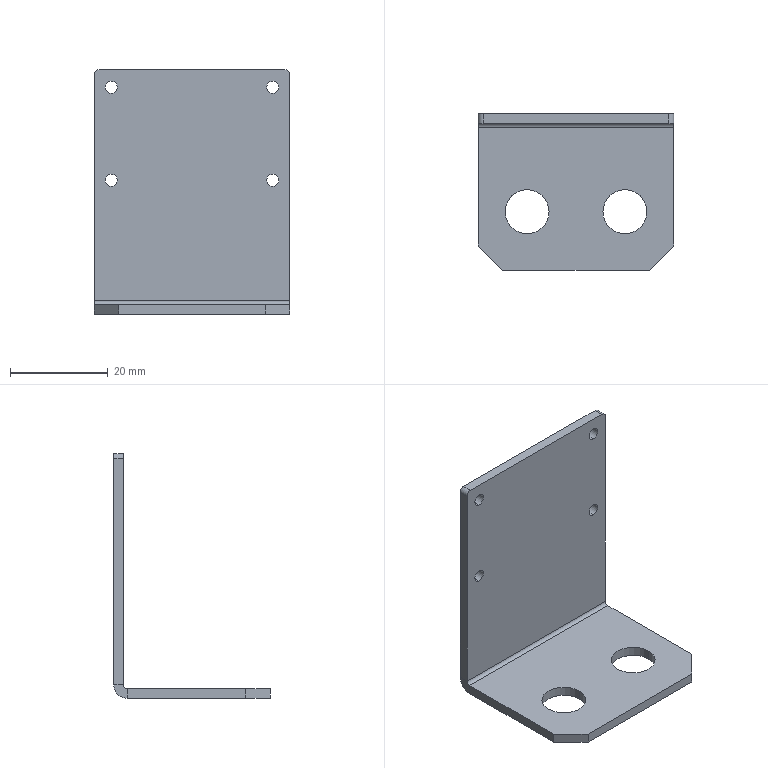Part | SolidWorks | features BaseBody 1 | 1 solid | 30 faces | box 40 x 32 x 50 mm | volume 5996 mm3 | cylinder 16 | plane 14 | commonest cylinder face diameters 2.5 x8 9 x4 2 x2 1.473 x1 5.473 x1
STEP:
#1=CARTESIAN_POINT('',(16.525,15.,24.15));
#2=VERTEX_POINT('',#1);
#3=CARTESIAN_POINT('',(16.525,15.,26.65));
#4=VERTEX_POINT('',#3);
#5=CARTESIAN_POINT('',(16.525,15.,25.4));
#6=DIRECTION('',(0.,1.,0.));
#7=DIRECTION('',(0.,0.,1.));
#8=AXIS2_PLACEMENT_3D('',#5,#6,#7);
#9=CIRCLE('',#8,1.25);
#10=EDGE_CURVE('',#2,#4,#9,.T.);
#11=ORIENTED_EDGE('',*,*,#10,.F.);
#12=CARTESIAN_POINT('',(16.525,17.,24.15));
#13=VERTEX_POINT('',#12);
#14=CARTESIAN_POINT('',(16.525,17.,24.15));
#15=DIRECTION('',(0.,1.,0.));
#16=VECTOR('',#15,1000.);
#17=LINE('',#14,#16);
#18=EDGE_CURVE('',#2,#13,#17,.T.);
#19=ORIENTED_EDGE('',*,*,#18,.T.);
#20=CARTESIAN_POINT('',(16.525,17.,26.65));
#21=VERTEX_POINT('',#20);
#22=CARTESIAN_POINT('',(16.525,17.,25.4));
#23=DIRECTION('',(0.,1.,0.));
#24=DIRECTION('',(0.,0.,1.));
#25=AXIS2_PLACEMENT_3D('',#22,#23,#24);
#26=CIRCLE('',#25,1.25);
#27=EDGE_CURVE('',#13,#21,#26,.T.);
#28=ORIENTED_EDGE('',*,*,#27,.T.);
#29=CARTESIAN_POINT('',(16.525,17.,26.65));
#30=DIRECTION('',(0.,1.,0.));
#31=VECTOR('',#30,1000.);
#32=LINE('',#29,#31);
#33=EDGE_CURVE('',#4,#21,#32,.T.);
#34=ORIENTED_EDGE('',*,*,#33,.F.);
#35=EDGE_LOOP('',(#11,#19,#28,#34));
#36=FACE_OUTER_BOUND('',#35,.T.);
#37=CARTESIAN_POINT('',(16.525,17.,25.4));
#38=DIRECTION('',(0.,1.,0.));
#39=DIRECTION('',(0.,0.,1.));
#40=AXIS2_PLACEMENT_3D('',#37,#38,#39);
#41=CYLINDRICAL_SURFACE('',#40,1.25);
#42=ADVANCED_FACE('',(#36),#41,.F.);
#43=CARTESIAN_POINT('',(16.525,15.,43.15));
#44=VERTEX_POINT('',#43);
#45=CARTESIAN_POINT('',(16.525,15.,45.65));
#46=VERTEX_POINT('',#45);
#47=CARTESIAN_POINT('',(16.525,15.,44.4));
#48=DIRECTION('',(0.,1.,0.));
#49=DIRECTION('',(0.,0.,1.));
#50=AXIS2_PLACEMENT_3D('',#47,#48,#49);
#51=CIRCLE('',#50,1.25);
#52=EDGE_CURVE('',#44,#46,#51,.T.);
#53=ORIENTED_EDGE('',*,*,#52,.F.);
#54=CARTESIAN_POINT('',(16.525,17.,43.15));
#55=VERTEX_POINT('',#54);
#56=CARTESIAN_POINT('',(16.525,17.,43.15));
#57=DIRECTION('',(0.,1.,0.));
#58=VECTOR('',#57,1000.);
#59=LINE('',#56,#58);
#60=EDGE_CURVE('',#44,#55,#59,.T.);
#61=ORIENTED_EDGE('',*,*,#60,.T.);
#62=CARTESIAN_POINT('',(16.525,17.,45.65));
#63=VERTEX_POINT('',#62);
#64=CARTESIAN_POINT('',(16.525,17.,44.4));
#65=DIRECTION('',(0.,1.,0.));
#66=DIRECTION('',(0.,0.,1.));
#67=AXIS2_PLACEMENT_3D('',#64,#65,#66);
#68=CIRCLE('',#67,1.25);
#69=EDGE_CURVE('',#55,#63,#68,.T.);
#70=ORIENTED_EDGE('',*,*,#69,.T.);
#71=CARTESIAN_POINT('',(16.525,17.,45.65));
#72=DIRECTION('',(0.,1.,0.));
#73=VECTOR('',#72,1000.);
#74=LINE('',#71,#73);
#75=EDGE_CURVE('',#46,#63,#74,.T.);
#76=ORIENTED_EDGE('',*,*,#75,.F.);
#77=EDGE_LOOP('',(#53,#61,#70,#76));
#78=FACE_OUTER_BOUND('',#77,.T.);
#79=CARTESIAN_POINT('',(16.525,17.,44.4));
#80=DIRECTION('',(0.,1.,0.));
#81=DIRECTION('',(0.,0.,1.));
#82=AXIS2_PLACEMENT_3D('',#79,#80,#81);
#83=CYLINDRICAL_SURFACE('',#82,1.25);
#84=ADVANCED_FACE('',(#78),#83,.F.);
#85=CARTESIAN_POINT('',(-16.525,15.,43.15));
#86=VERTEX_POINT('',#85);
#87=CARTESIAN_POINT('',(-16.525,15.,45.65));
#88=VERTEX_POINT('',#87);
#89=CARTESIAN_POINT('',(-16.525,15.,44.4));
#90=DIRECTION('',(0.,1.,0.));
#91=DIRECTION('',(0.,0.,1.));
#92=AXIS2_PLACEMENT_3D('',#89,#90,#91);
#93=CIRCLE('',#92,1.25);
#94=EDGE_CURVE('',#86,#88,#93,.T.);
#95=ORIENTED_EDGE('',*,*,#94,.F.);
#96=CARTESIAN_POINT('',(-16.525,17.,43.15));
#97=VERTEX_POINT('',#96);
#98=CARTESIAN_POINT('',(-16.525,17.,43.15));
#99=DIRECTION('',(0.,1.,0.));
#100=VECTOR('',#99,1000.);
#101=LINE('',#98,#100);
#102=EDGE_CURVE('',#86,#97,#101,.T.);
#103=ORIENTED_EDGE('',*,*,#102,.T.);
#104=CARTESIAN_POINT('',(-16.525,17.,45.65));
#105=VERTEX_POINT('',#104);
#106=CARTESIAN_POINT('',(-16.525,17.,44.4));
#107=DIRECTION('',(0.,1.,0.));
#108=DIRECTION('',(0.,0.,1.));
#109=AXIS2_PLACEMENT_3D('',#106,#107,#108);
#110=CIRCLE('',#109,1.25);
#111=EDGE_CURVE('',#97,#105,#110,.T.);
#112=ORIENTED_EDGE('',*,*,#111,.T.);
#113=CARTESIAN_POINT('',(-16.525,17.,45.65));
#114=DIRECTION('',(0.,1.,0.));
#115=VECTOR('',#114,1000.);
#116=LINE('',#113,#115);
#117=EDGE_CURVE('',#88,#105,#116,.T.);
#118=ORIENTED_EDGE('',*,*,#117,.F.);
#119=EDGE_LOOP('',(#95,#103,#112,#118));
#120=FACE_OUTER_BOUND('',#119,.T.);
#121=CARTESIAN_POINT('',(-16.525,17.,44.4));
#122=DIRECTION('',(0.,1.,0.));
#123=DIRECTION('',(0.,0.,1.));
#124=AXIS2_PLACEMENT_3D('',#121,#122,#123);
#125=CYLINDRICAL_SURFACE('',#124,1.25);
#126=ADVANCED_FACE('',(#120),#125,.F.);
#127=CARTESIAN_POINT('',(-16.525,15.,24.15));
#128=VERTEX_POINT('',#127);
#129=CARTESIAN_POINT('',(-16.525,15.,26.65));
#130=VERTEX_POINT('',#129);
#131=CARTESIAN_POINT('',(-16.525,15.,25.4));
#132=DIRECTION('',(0.,1.,0.));
#133=DIRECTION('',(0.,0.,1.));
#134=AXIS2_PLACEMENT_3D('',#131,#132,#133);
#135=CIRCLE('',#134,1.25);
#136=EDGE_CURVE('',#128,#130,#135,.T.);
#137=ORIENTED_EDGE('',*,*,#136,.F.);
#138=CARTESIAN_POINT('',(-16.525,17.,24.15));
#139=VERTEX_POINT('',#138);
#140=CARTESIAN_POINT('',(-16.525,17.,24.15));
#141=DIRECTION('',(0.,1.,0.));
#142=VECTOR('',#141,1000.);
#143=LINE('',#140,#142);
#144=EDGE_CURVE('',#128,#139,#143,.T.);
#145=ORIENTED_EDGE('',*,*,#144,.T.);
#146=CARTESIAN_POINT('',(-16.525,17.,26.65));
#147=VERTEX_POINT('',#146);
#148=CARTESIAN_POINT('',(-16.525,17.,25.4));
#149=DIRECTION('',(0.,1.,0.));
#150=DIRECTION('',(0.,0.,1.));
#151=AXIS2_PLACEMENT_3D('',#148,#149,#150);
#152=CIRCLE('',#151,1.25);
#153=EDGE_CURVE('',#139,#147,#152,.T.);
#154=ORIENTED_EDGE('',*,*,#153,.T.);
#155=CARTESIAN_POINT('',(-16.525,17.,26.65));
#156=DIRECTION('',(0.,1.,0.));
#157=VECTOR('',#156,1000.);
#158=LINE('',#155,#157);
#159=EDGE_CURVE('',#130,#147,#158,.T.);
#160=ORIENTED_EDGE('',*,*,#159,.F.);
#161=EDGE_LOOP('',(#137,#145,#154,#160));
#162=FACE_OUTER_BOUND('',#161,.T.);
#163=CARTESIAN_POINT('',(-16.525,17.,25.4));
#164=DIRECTION('',(0.,1.,0.));
#165=DIRECTION('',(0.,0.,1.));
#166=AXIS2_PLACEMENT_3D('',#163,#164,#165);
#167=CYLINDRICAL_SURFACE('',#166,1.25);
#168=ADVANCED_FACE('',(#162),#167,.F.);
#169=CARTESIAN_POINT('',(-14.5,-3.,-2.));
#170=VERTEX_POINT('',#169);
#171=CARTESIAN_POINT('',(-5.5,-3.,-2.));
#172=VERTEX_POINT('',#171);
#173=CARTESIAN_POINT('',(-10.,-3.,-2.));
#174=DIRECTION('',(0.,0.,1.));
#175=DIRECTION('',(1.,0.,0.));
#176=AXIS2_PLACEMENT_3D('',#173,#174,#175);
#177=CIRCLE('',#176,4.5);
#178=EDGE_CURVE('',#170,#172,#177,.T.);
#179=ORIENTED_EDGE('',*,*,#178,.F.);
#180=CARTESIAN_POINT('',(-14.5,-3.,0.));
#181=VERTEX_POINT('',#180);
#182=CARTESIAN_POINT('',(-14.5,-3.,0.));
#183=DIRECTION('',(0.,0.,1.));
#184=VECTOR('',#183,1000.);
#185=LINE('',#182,#184);
#186=EDGE_CURVE('',#170,#181,#185,.T.);
#187=ORIENTED_EDGE('',*,*,#186,.T.);
#188=CARTESIAN_POINT('',(-5.5,-3.,0.));
#189=VERTEX_POINT('',#188);
#190=CARTESIAN_POINT('',(-10.,-3.,0.));
#191=DIRECTION('',(0.,0.,1.));
#192=DIRECTION('',(1.,0.,0.));
#193=AXIS2_PLACEMENT_3D('',#190,#191,#192);
#194=CIRCLE('',#193,4.5);
#195=EDGE_CURVE('',#181,#189,#194,.T.);
#196=ORIENTED_EDGE('',*,*,#195,.T.);
#197=CARTESIAN_POINT('',(-5.5,-3.,0.));
#198=DIRECTION('',(0.,0.,1.));
#199=VECTOR('',#198,1000.);
#200=LINE('',#197,#199);
#201=EDGE_CURVE('',#172,#189,#200,.T.);
#202=ORIENTED_EDGE('',*,*,#201,.F.);
#203=EDGE_LOOP('',(#179,#187,#196,#202));
#204=FACE_OUTER_BOUND('',#203,.T.);
#205=CARTESIAN_POINT('',(-10.,-3.,0.));
#206=DIRECTION('',(0.,0.,1.));
#207=DIRECTION('',(1.,0.,0.));
#208=AXIS2_PLACEMENT_3D('',#205,#206,#207);
#209=CYLINDRICAL_SURFACE('',#208,4.5);
#210=ADVANCED_FACE('',(#204),#209,.F.);
#211=CARTESIAN_POINT('',(5.5,-3.,-2.));
#212=VERTEX_POINT('',#211);
#213=CARTESIAN_POINT('',(14.5,-3.,-2.));
#214=VERTEX_POINT('',#213);
#215=CARTESIAN_POINT('',(10.,-3.,-2.));
#216=DIRECTION('',(0.,0.,1.));
#217=DIRECTION('',(1.,0.,0.));
#218=AXIS2_PLACEMENT_3D('',#215,#216,#217);
#219=CIRCLE('',#218,4.5);
#220=EDGE_CURVE('',#212,#214,#219,.T.);
#221=ORIENTED_EDGE('',*,*,#220,.F.);
#222=CARTESIAN_POINT('',(5.5,-3.,0.));
#223=VERTEX_POINT('',#222);
#224=CARTESIAN_POINT('',(5.5,-3.,0.));
#225=DIRECTION('',(0.,0.,1.));
#226=VECTOR('',#225,1000.);
#227=LINE('',#224,#226);
#228=EDGE_CURVE('',#212,#223,#227,.T.);
#229=ORIENTED_EDGE('',*,*,#228,.T.);
#230=CARTESIAN_POINT('',(14.5,-3.,0.));
#231=VERTEX_POINT('',#230);
#232=CARTESIAN_POINT('',(10.,-3.,0.));
#233=DIRECTION('',(0.,0.,1.));
#234=DIRECTION('',(1.,0.,0.));
#235=AXIS2_PLACEMENT_3D('',#232,#233,#234);
#236=CIRCLE('',#235,4.5);
#237=EDGE_CURVE('',#223,#231,#236,.T.);
#238=ORIENTED_EDGE('',*,*,#237,.T.);
#239=CARTESIAN_POINT('',(14.5,-3.,0.));
#240=DIRECTION('',(0.,0.,1.));
#241=VECTOR('',#240,1000.);
#242=LINE('',#239,#241);
#243=EDGE_CURVE('',#214,#231,#242,.T.);
#244=ORIENTED_EDGE('',*,*,#243,.F.);
#245=EDGE_LOOP('',(#221,#229,#238,#244));
#246=FACE_OUTER_BOUND('',#245,.T.);
#247=CARTESIAN_POINT('',(10.,-3.,0.));
#248=DIRECTION('',(0.,0.,1.));
#249=DIRECTION('',(1.,0.,0.));
#250=AXIS2_PLACEMENT_3D('',#247,#248,#249);
#251=CYLINDRICAL_SURFACE('',#250,4.5);
#252=ADVANCED_FACE('',(#246),#251,.F.);
#253=CARTESIAN_POINT('',(-20.,14.263,-2.));
#254=VERTEX_POINT('',#253);
#255=CARTESIAN_POINT('',(-20.,-10.,-2.));
#256=VERTEX_POINT('',#255);
#257=CARTESIAN_POINT('',(-20.,15.,-2.));
#258=DIRECTION('',(0.,-1.,0.));
#259=VECTOR('',#258,1000.);
#260=LINE('',#257,#259);
#261=EDGE_CURVE('',#254,#256,#260,.T.);
#262=ORIENTED_EDGE('',*,*,#261,.T.);
#263=CARTESIAN_POINT('',(-20.,-10.,0.));
#264=VERTEX_POINT('',#263);
#265=CARTESIAN_POINT('',(-20.,-10.,-2.));
#266=DIRECTION('',(0.,0.,1.));
#267=VECTOR('',#266,1000.);
#268=LINE('',#265,#267);
#269=EDGE_CURVE('',#256,#264,#268,.T.);
#270=ORIENTED_EDGE('',*,*,#269,.T.);
#271=CARTESIAN_POINT('',(-20.,14.263,0.));
#272=VERTEX_POINT('',#271);
#273=CARTESIAN_POINT('',(-20.,15.,0.));
#274=DIRECTION('',(0.,-1.,0.));
#275=VECTOR('',#274,1000.);
#276=LINE('',#273,#275);
#277=EDGE_CURVE('',#272,#264,#276,.T.);
#278=ORIENTED_EDGE('',*,*,#277,.F.);
#279=CARTESIAN_POINT('',(-20.,14.263,0.));
#280=DIRECTION('',(0.,0.,-1.));
#281=VECTOR('',#280,1000.);
#282=LINE('',#279,#281);
#283=EDGE_CURVE('',#272,#254,#282,.T.);
#284=ORIENTED_EDGE('',*,*,#283,.T.);
#285=EDGE_LOOP('',(#262,#270,#278,#284));
#286=FACE_OUTER_BOUND('',#285,.T.);
#287=CARTESIAN_POINT('',(-20.,15.,-2.));
#288=DIRECTION('',(-1.,0.,0.));
#289=DIRECTION('',(0.,-1.,0.));
#290=AXIS2_PLACEMENT_3D('',#287,#288,#289);
#291=PLANE('',#290);
#292=ADVANCED_FACE('',(#286),#291,.T.);
#293=CARTESIAN_POINT('',(-10.,-3.,-2.));
#294=DIRECTION('',(0.,0.,1.));
#295=DIRECTION('',(1.,0.,0.));
#296=AXIS2_PLACEMENT_3D('',#293,#294,#295);
#297=CIRCLE('',#296,4.5);
#298=EDGE_CURVE('',#172,#170,#297,.T.);
#299=ORIENTED_EDGE('',*,*,#298,.T.);
#300=ORIENTED_EDGE('',*,*,#178,.T.);
#301=EDGE_LOOP('',(#299,#300));
#302=FACE_BOUND('',#301,.T.);
#303=CARTESIAN_POINT('',(10.,-3.,-2.));
#304=DIRECTION('',(0.,0.,1.));
#305=DIRECTION('',(1.,0.,0.));
#306=AXIS2_PLACEMENT_3D('',#303,#304,#305);
#307=CIRCLE('',#306,4.5);
#308=EDGE_CURVE('',#214,#212,#307,.T.);
#309=ORIENTED_EDGE('',*,*,#308,.T.);
#310=ORIENTED_EDGE('',*,*,#220,.T.);
#311=EDGE_LOOP('',(#309,#310));
#312=FACE_BOUND('',#311,.T.);
#313=CARTESIAN_POINT('',(20.,-10.,-2.));
#314=VERTEX_POINT('',#313);
#315=CARTESIAN_POINT('',(20.,14.263,-2.));
#316=VERTEX_POINT('',#315);
#317=CARTESIAN_POINT('',(20.,15.,-2.));
#318=DIRECTION('',(0.,1.,0.));
#319=VECTOR('',#318,1000.);
#320=LINE('',#317,#319);
#321=EDGE_CURVE('',#314,#316,#320,.T.);
#322=ORIENTED_EDGE('',*,*,#321,.F.);
#323=CARTESIAN_POINT('',(15.,-15.,-2.));
#324=VERTEX_POINT('',#323);
#325=CARTESIAN_POINT('',(15.,-15.,-2.));
#326=DIRECTION('',(-0.7071,-0.7071,0.));
#327=VECTOR('',#326,1000.);
#328=LINE('',#325,#327);
#329=EDGE_CURVE('',#314,#324,#328,.T.);
#330=ORIENTED_EDGE('',*,*,#329,.T.);
#331=CARTESIAN_POINT('',(-15.,-15.,-2.));
#332=VERTEX_POINT('',#331);
#333=CARTESIAN_POINT('',(20.,-15.,-2.));
#334=DIRECTION('',(1.,0.,0.));
#335=VECTOR('',#334,1000.);
#336=LINE('',#333,#335);
#337=EDGE_CURVE('',#332,#324,#336,.T.);
#338=ORIENTED_EDGE('',*,*,#337,.F.);
#339=CARTESIAN_POINT('',(-15.,-15.,-2.));
#340=DIRECTION('',(-0.7071,0.7071,0.));
#341=VECTOR('',#340,1000.);
#342=LINE('',#339,#341);
#343=EDGE_CURVE('',#332,#256,#342,.T.);
#344=ORIENTED_EDGE('',*,*,#343,.T.);
#345=ORIENTED_EDGE('',*,*,#261,.F.);
#346=CARTESIAN_POINT('',(-20.,14.263,-2.));
#347=DIRECTION('',(1.,0.,0.));
#348=VECTOR('',#347,1000.);
#349=LINE('',#346,#348);
#350=EDGE_CURVE('',#254,#316,#349,.T.);
#351=ORIENTED_EDGE('',*,*,#350,.T.);
#352=EDGE_LOOP('',(#322,#330,#338,#344,#345,#351));
#353=FACE_OUTER_BOUND('',#352,.T.);
#354=CARTESIAN_POINT('',(0.,0.,-2.));
#355=DIRECTION('',(0.,0.,-1.));
#356=DIRECTION('',(-1.,0.,0.));
#357=AXIS2_PLACEMENT_3D('',#354,#355,#356);
#358=PLANE('',#357);
#359=ADVANCED_FACE('',(#302,#312,#353),#358,.T.);
#360=CARTESIAN_POINT('',(-10.,-3.,0.));
#361=DIRECTION('',(0.,0.,1.));
#362=DIRECTION('',(1.,0.,0.));
#363=AXIS2_PLACEMENT_3D('',#360,#361,#362);
#364=CIRCLE('',#363,4.5);
#365=EDGE_CURVE('',#189,#181,#364,.T.);
#366=ORIENTED_EDGE('',*,*,#365,.F.);
#367=ORIENTED_EDGE('',*,*,#195,.F.);
#368=EDGE_LOOP('',(#366,#367));
#369=FACE_BOUND('',#368,.T.);
#370=CARTESIAN_POINT('',(10.,-3.,0.));
#371=DIRECTION('',(0.,0.,1.));
#372=DIRECTION('',(1.,0.,0.));
#373=AXIS2_PLACEMENT_3D('',#370,#371,#372);
#374=CIRCLE('',#373,4.5);
#375=EDGE_CURVE('',#231,#223,#374,.T.);
#376=ORIENTED_EDGE('',*,*,#375,.F.);
#377=ORIENTED_EDGE('',*,*,#237,.F.);
#378=EDGE_LOOP('',(#376,#377));
#379=FACE_BOUND('',#378,.T.);
#380=CARTESIAN_POINT('',(-15.,-15.,0.));
#381=VERTEX_POINT('',#380);
#382=CARTESIAN_POINT('',(15.,-15.,0.));
#383=VERTEX_POINT('',#382);
#384=CARTESIAN_POINT('',(20.,-15.,0.));
#385=DIRECTION('',(1.,0.,0.));
#386=VECTOR('',#385,1000.);
#387=LINE('',#384,#386);
#388=EDGE_CURVE('',#381,#383,#387,.T.);
#389=ORIENTED_EDGE('',*,*,#388,.T.);
#390=CARTESIAN_POINT('',(20.,-10.,0.));
#391=VERTEX_POINT('',#390);
#392=CARTESIAN_POINT('',(15.,-15.,0.));
#393=DIRECTION('',(0.7071,0.7071,0.));
#394=VECTOR('',#393,1000.);
#395=LINE('',#392,#394);
#396=EDGE_CURVE('',#383,#391,#395,.T.);
#397=ORIENTED_EDGE('',*,*,#396,.T.);
#398=CARTESIAN_POINT('',(20.,14.263,0.));
#399=VERTEX_POINT('',#398);
#400=CARTESIAN_POINT('',(20.,15.,0.));
#401=DIRECTION('',(0.,1.,0.));
#402=VECTOR('',#401,1000.);
#403=LINE('',#400,#402);
#404=EDGE_CURVE('',#391,#399,#403,.T.);
#405=ORIENTED_EDGE('',*,*,#404,.T.);
#406=CARTESIAN_POINT('',(-20.,14.263,0.));
#407=DIRECTION('',(1.,0.,0.));
#408=VECTOR('',#407,1000.);
#409=LINE('',#406,#408);
#410=EDGE_CURVE('',#272,#399,#409,.T.);
#411=ORIENTED_EDGE('',*,*,#410,.F.);
#412=ORIENTED_EDGE('',*,*,#277,.T.);
#413=CARTESIAN_POINT('',(-20.,-10.,0.));
#414=DIRECTION('',(0.7071,-0.7071,0.));
#415=VECTOR('',#414,1000.);
#416=LINE('',#413,#415);
#417=EDGE_CURVE('',#264,#381,#416,.T.);
#418=ORIENTED_EDGE('',*,*,#417,.T.);
#419=EDGE_LOOP('',(#389,#397,#405,#411,#412,#418));
#420=FACE_OUTER_BOUND('',#419,.T.);
#421=CARTESIAN_POINT('',(0.,0.,0.));
#422=DIRECTION('',(0.,0.,-1.));
#423=DIRECTION('',(-1.,0.,0.));
#424=AXIS2_PLACEMENT_3D('',#421,#422,#423);
#425=PLANE('',#424);
#426=ADVANCED_FACE('',(#369,#379,#420),#425,.F.);
#427=ORIENTED_EDGE('',*,*,#404,.F.);
#428=CARTESIAN_POINT('',(20.,-10.,-2.));
#429=DIRECTION('',(0.,0.,-1.));
#430=VECTOR('',#429,1000.);
#431=LINE('',#428,#430);
#432=EDGE_CURVE('',#391,#314,#431,.T.);
#433=ORIENTED_EDGE('',*,*,#432,.T.);
#434=ORIENTED_EDGE('',*,*,#321,.T.);
#435=CARTESIAN_POINT('',(20.,14.263,0.));
#436=DIRECTION('',(0.,0.,-1.));
#437=VECTOR('',#436,1000.);
#438=LINE('',#435,#437);
#439=EDGE_CURVE('',#399,#316,#438,.T.);
#440=ORIENTED_EDGE('',*,*,#439,.F.);
#441=EDGE_LOOP('',(#427,#433,#434,#440));
#442=FACE_OUTER_BOUND('',#441,.T.);
#443=CARTESIAN_POINT('',(20.,15.,-2.));
#444=DIRECTION('',(1.,0.,0.));
#445=DIRECTION('',(0.,1.,0.));
#446=AXIS2_PLACEMENT_3D('',#443,#444,#445);
#447=PLANE('',#446);
#448=ADVANCED_FACE('',(#442),#447,.T.);
#449=ORIENTED_EDGE('',*,*,#337,.T.);
#450=CARTESIAN_POINT('',(15.,-15.,-2.));
#451=DIRECTION('',(0.,0.,1.));
#452=VECTOR('',#451,1000.);
#453=LINE('',#450,#452);
#454=EDGE_CURVE('',#324,#383,#453,.T.);
#455=ORIENTED_EDGE('',*,*,#454,.T.);
#456=ORIENTED_EDGE('',*,*,#388,.F.);
#457=CARTESIAN_POINT('',(-15.,-15.,-2.));
#458=DIRECTION('',(0.,0.,-1.));
#459=VECTOR('',#458,1000.);
#460=LINE('',#457,#459);
#461=EDGE_CURVE('',#381,#332,#460,.T.);
#462=ORIENTED_EDGE('',*,*,#461,.T.);
#463=EDGE_LOOP('',(#449,#455,#456,#462));
#464=FACE_OUTER_BOUND('',#463,.T.);
#465=CARTESIAN_POINT('',(20.,-15.,-2.));
#466=DIRECTION('',(0.,-1.,0.));
#467=DIRECTION('',(1.,0.,0.));
#468=AXIS2_PLACEMENT_3D('',#465,#466,#467);
#469=PLANE('',#468);
#470=ADVANCED_FACE('',(#464),#469,.T.);
#471=CARTESIAN_POINT('',(20.,15.,0.7366));
#472=VERTEX_POINT('',#471);
#473=CARTESIAN_POINT('',(20.,17.,0.7366));
#474=VERTEX_POINT('',#473);
#475=CARTESIAN_POINT('',(20.,15.,0.7366));
#476=DIRECTION('',(0.,1.,0.));
#477=VECTOR('',#476,1000.);
#478=LINE('',#475,#477);
#479=EDGE_CURVE('',#472,#474,#478,.T.);
#480=ORIENTED_EDGE('',*,*,#479,.F.);
#481=CARTESIAN_POINT('',(20.,14.263,0.7366));
#482=DIRECTION('',(1.,0.,0.));
#483=DIRECTION('',(0.,0.,1.));
#484=AXIS2_PLACEMENT_3D('',#481,#482,#483);
#485=CIRCLE('',#484,0.7366);
#486=EDGE_CURVE('',#399,#472,#485,.T.);
#487=ORIENTED_EDGE('',*,*,#486,.F.);
#488=ORIENTED_EDGE('',*,*,#439,.T.);
#489=CARTESIAN_POINT('',(20.,14.263,0.7366));
#490=DIRECTION('',(1.,0.,0.));
#491=DIRECTION('',(0.,0.,1.));
#492=AXIS2_PLACEMENT_3D('',#489,#490,#491);
#493=CIRCLE('',#492,2.737);
#494=EDGE_CURVE('',#316,#474,#493,.T.);
#495=ORIENTED_EDGE('',*,*,#494,.T.);
#496=EDGE_LOOP('',(#480,#487,#488,#495));
#497=FACE_OUTER_BOUND('',#496,.T.);
#498=CARTESIAN_POINT('',(20.,14.263,0.7366));
#499=DIRECTION('',(1.,0.,0.));
#500=DIRECTION('',(0.,0.,-1.));
#501=AXIS2_PLACEMENT_3D('',#498,#499,#500);
#502=PLANE('',#501);
#503=ADVANCED_FACE('',(#497),#502,.T.);
#504=CARTESIAN_POINT('',(-20.,15.,0.7366));
#505=VERTEX_POINT('',#504);
#506=CARTESIAN_POINT('',(-20.,14.263,0.7366));
#507=DIRECTION('',(-1.,0.,0.));
#508=DIRECTION('',(0.,0.,1.));
#509=AXIS2_PLACEMENT_3D('',#506,#507,#508);
#510=CIRCLE('',#509,0.7366);
#511=EDGE_CURVE('',#505,#272,#510,.T.);
#512=ORIENTED_EDGE('',*,*,#511,.F.);
#513=CARTESIAN_POINT('',(-20.,17.,0.7366));
#514=VERTEX_POINT('',#513);
#515=CARTESIAN_POINT('',(-20.,15.,0.7366));
#516=DIRECTION('',(0.,1.,0.));
#517=VECTOR('',#516,1000.);
#518=LINE('',#515,#517);
#519=EDGE_CURVE('',#505,#514,#518,.T.);
#520=ORIENTED_EDGE('',*,*,#519,.T.);
#521=CARTESIAN_POINT('',(-20.,14.263,0.7366));
#522=DIRECTION('',(-1.,0.,0.));
#523=DIRECTION('',(0.,0.,1.));
#524=AXIS2_PLACEMENT_3D('',#521,#522,#523);
#525=CIRCLE('',#524,2.737);
#526=EDGE_CURVE('',#514,#254,#525,.T.);
#527=ORIENTED_EDGE('',*,*,#526,.T.);
#528=ORIENTED_EDGE('',*,*,#283,.F.);
#529=EDGE_LOOP('',(#512,#520,#527,#528));
#530=FACE_OUTER_BOUND('',#529,.T.);
#531=CARTESIAN_POINT('',(-20.,14.263,0.7366));
#532=DIRECTION('',(1.,0.,0.));
#533=DIRECTION('',(0.,0.,-1.));
#534=AXIS2_PLACEMENT_3D('',#531,#532,#533);
#535=PLANE('',#534);
#536=ADVANCED_FACE('',(#530),#535,.F.);
#537=ORIENTED_EDGE('',*,*,#350,.F.);
#538=ORIENTED_EDGE('',*,*,#526,.F.);
#539=CARTESIAN_POINT('',(0.,17.,0.7366));
#540=DIRECTION('',(-1.,0.,0.));
#541=VECTOR('',#540,1000.);
#542=LINE('',#539,#541);
#543=EDGE_CURVE('',#474,#514,#542,.T.);
#544=ORIENTED_EDGE('',*,*,#543,.F.);
#545=ORIENTED_EDGE('',*,*,#494,.F.);
#546=EDGE_LOOP('',(#537,#538,#544,#545));
#547=FACE_OUTER_BOUND('',#546,.T.);
#548=CARTESIAN_POINT('',(-20.,14.263,0.7366));
#549=DIRECTION('',(-1.,0.,0.));
#550=DIRECTION('',(0.,1.,0.));
#551=AXIS2_PLACEMENT_3D('',#548,#549,#550);
#552=CYLINDRICAL_SURFACE('',#551,2.737);
#553=ADVANCED_FACE('',(#547),#552,.T.);
#554=ORIENTED_EDGE('',*,*,#410,.T.);
#555=ORIENTED_EDGE('',*,*,#486,.T.);
#556=CARTESIAN_POINT('',(20.,15.,0.7366));
#557=DIRECTION('',(-1.,0.,0.));
#558=VECTOR('',#557,1000.);
#559=LINE('',#556,#558);
#560=EDGE_CURVE('',#472,#505,#559,.T.);
#561=ORIENTED_EDGE('',*,*,#560,.T.);
#562=ORIENTED_EDGE('',*,*,#511,.T.);
#563=EDGE_LOOP('',(#554,#555,#561,#562));
#564=FACE_OUTER_BOUND('',#563,.T.);
#565=CARTESIAN_POINT('',(-20.,14.263,0.7366));
#566=DIRECTION('',(-1.,0.,0.));
#567=DIRECTION('',(0.,1.,0.));
#568=AXIS2_PLACEMENT_3D('',#565,#566,#567);
#569=CYLINDRICAL_SURFACE('',#568,0.7366);
#570=ADVANCED_FACE('',(#564),#569,.F.);
#571=CARTESIAN_POINT('',(-20.,15.,47.));
#572=VERTEX_POINT('',#571);
#573=CARTESIAN_POINT('',(-20.,15.,0.));
#574=DIRECTION('',(0.,0.,-1.));
#575=VECTOR('',#574,1000.);
#576=LINE('',#573,#575);
#577=EDGE_CURVE('',#572,#505,#576,.T.);
#578=ORIENTED_EDGE('',*,*,#577,.F.);
#579=CARTESIAN_POINT('',(-20.,17.,47.));
#580=VERTEX_POINT('',#579);
#581=CARTESIAN_POINT('',(-20.,17.,47.));
#582=DIRECTION('',(0.,1.,0.));
#583=VECTOR('',#582,1000.);
#584=LINE('',#581,#583);
#585=EDGE_CURVE('',#572,#580,#584,.T.);
#586=ORIENTED_EDGE('',*,*,#585,.T.);
#587=CARTESIAN_POINT('',(-20.,17.,0.));
#588=DIRECTION('',(0.,0.,-1.));
#589=VECTOR('',#588,1000.);
#590=LINE('',#587,#589);
#591=EDGE_CURVE('',#580,#514,#590,.T.);
#592=ORIENTED_EDGE('',*,*,#591,.T.);
#593=ORIENTED_EDGE('',*,*,#519,.F.);
#594=EDGE_LOOP('',(#578,#586,#592,#593));
#595=FACE_OUTER_BOUND('',#594,.T.);
#596=CARTESIAN_POINT('',(-20.,17.,0.));
#597=DIRECTION('',(-1.,0.,0.));
#598=DIRECTION('',(0.,-1.,0.));
#599=AXIS2_PLACEMENT_3D('',#596,#597,#598);
#600=PLANE('',#599);
#601=ADVANCED_FACE('',(#595),#600,.T.);
#602=CARTESIAN_POINT('',(20.,17.,47.));
#603=VERTEX_POINT('',#602);
#604=CARTESIAN_POINT('',(20.,17.,48.));
#605=DIRECTION('',(0.,0.,1.));
#606=VECTOR('',#605,1000.);
#607=LINE('',#604,#606);
#608=EDGE_CURVE('',#474,#603,#607,.T.);
#609=ORIENTED_EDGE('',*,*,#608,.T.);
#610=CARTESIAN_POINT('',(20.,15.,47.));
#611=VERTEX_POINT('',#610);
#612=CARTESIAN_POINT('',(20.,17.,47.));
#613=DIRECTION('',(0.,-1.,0.));
#614=VECTOR('',#613,1000.);
#615=LINE('',#612,#614);
#616=EDGE_CURVE('',#603,#611,#615,.T.);
#617=ORIENTED_EDGE('',*,*,#616,.T.);
#618=CARTESIAN_POINT('',(20.,15.,48.));
#619=DIRECTION('',(0.,0.,1.));
#620=VECTOR('',#619,1000.);
#621=LINE('',#618,#620);
#622=EDGE_CURVE('',#472,#611,#621,.T.);
#623=ORIENTED_EDGE('',*,*,#622,.F.);
#624=ORIENTED_EDGE('',*,*,#479,.T.);
#625=EDGE_LOOP('',(#609,#617,#623,#624));
#626=FACE_OUTER_BOUND('',#625,.T.);
#627=CARTESIAN_POINT('',(20.,17.,48.));
#628=DIRECTION('',(1.,0.,0.));
#629=DIRECTION('',(0.,1.,0.));
#630=AXIS2_PLACEMENT_3D('',#627,#628,#629);
#631=PLANE('',#630);
#632=ADVANCED_FACE('',(#626),#631,.T.);
#633=CARTESIAN_POINT('',(16.525,17.,25.4));
#634=DIRECTION('',(0.,1.,0.));
#635=DIRECTION('',(0.,0.,1.));
#636=AXIS2_PLACEMENT_3D('',#633,#634,#635);
#637=CIRCLE('',#636,1.25);
#638=EDGE_CURVE('',#21,#13,#637,.T.);
#639=ORIENTED_EDGE('',*,*,#638,.F.);
#640=ORIENTED_EDGE('',*,*,#27,.F.);
#641=EDGE_LOOP('',(#639,#640));
#642=FACE_BOUND('',#641,.T.);
#643=CARTESIAN_POINT('',(16.525,17.,44.4));
#644=DIRECTION('',(0.,1.,0.));
#645=DIRECTION('',(0.,0.,1.));
#646=AXIS2_PLACEMENT_3D('',#643,#644,#645);
#647=CIRCLE('',#646,1.25);
#648=EDGE_CURVE('',#63,#55,#647,.T.);
#649=ORIENTED_EDGE('',*,*,#648,.F.);
#650=ORIENTED_EDGE('',*,*,#69,.F.);
#651=EDGE_LOOP('',(#649,#650));
#652=FACE_BOUND('',#651,.T.);
#653=CARTESIAN_POINT('',(-16.525,17.,44.4));
#654=DIRECTION('',(0.,1.,0.));
#655=DIRECTION('',(0.,0.,1.));
#656=AXIS2_PLACEMENT_3D('',#653,#654,#655);
#657=CIRCLE('',#656,1.25);
#658=EDGE_CURVE('',#105,#97,#657,.T.);
#659=ORIENTED_EDGE('',*,*,#658,.F.);
#660=ORIENTED_EDGE('',*,*,#111,.F.);
#661=EDGE_LOOP('',(#659,#660));
#662=FACE_BOUND('',#661,.T.);
#663=CARTESIAN_POINT('',(-16.525,17.,25.4));
#664=DIRECTION('',(0.,1.,0.));
#665=DIRECTION('',(0.,0.,1.));
#666=AXIS2_PLACEMENT_3D('',#663,#664,#665);
#667=CIRCLE('',#666,1.25);
#668=EDGE_CURVE('',#147,#139,#667,.T.);
#669=ORIENTED_EDGE('',*,*,#668,.F.);
#670=ORIENTED_EDGE('',*,*,#153,.F.);
#671=EDGE_LOOP('',(#669,#670));
#672=FACE_BOUND('',#671,.T.);
#673=CARTESIAN_POINT('',(19.,17.,48.));
#674=VERTEX_POINT('',#673);
#675=CARTESIAN_POINT('',(-19.,17.,48.));
#676=VERTEX_POINT('',#675);
#677=CARTESIAN_POINT('',(-20.,17.,48.));
#678=DIRECTION('',(-1.,0.,0.));
#679=VECTOR('',#678,1000.);
#680=LINE('',#677,#679);
#681=EDGE_CURVE('',#674,#676,#680,.T.);
#682=ORIENTED_EDGE('',*,*,#681,.F.);
#683=CARTESIAN_POINT('',(19.,17.,47.));
#684=DIRECTION('',(0.,1.,0.));
#685=DIRECTION('',(0.,0.,1.));
#686=AXIS2_PLACEMENT_3D('',#683,#684,#685);
#687=CIRCLE('',#686,1.);
#688=EDGE_CURVE('',#674,#603,#687,.T.);
#689=ORIENTED_EDGE('',*,*,#688,.T.);
#690=ORIENTED_EDGE('',*,*,#608,.F.);
#691=ORIENTED_EDGE('',*,*,#543,.T.);
#692=ORIENTED_EDGE('',*,*,#591,.F.);
#693=CARTESIAN_POINT('',(-19.,17.,47.));
#694=DIRECTION('',(0.,1.,0.));
#695=DIRECTION('',(0.,0.,1.));
#696=AXIS2_PLACEMENT_3D('',#693,#694,#695);
#697=CIRCLE('',#696,1.);
#698=EDGE_CURVE('',#580,#676,#697,.T.);
#699=ORIENTED_EDGE('',*,*,#698,.T.);
#700=EDGE_LOOP('',(#682,#689,#690,#691,#692,#699));
#701=FACE_OUTER_BOUND('',#700,.T.);
#702=CARTESIAN_POINT('',(0.,17.,0.));
#703=DIRECTION('',(0.,1.,0.));
#704=DIRECTION('',(0.,0.,1.));
#705=AXIS2_PLACEMENT_3D('',#702,#703,#704);
#706=PLANE('',#705);
#707=ADVANCED_FACE('',(#642,#652,#662,#672,#701),#706,.T.);
#708=CARTESIAN_POINT('',(16.525,15.,25.4));
#709=DIRECTION('',(0.,1.,0.));
#710=DIRECTION('',(0.,0.,1.));
#711=AXIS2_PLACEMENT_3D('',#708,#709,#710);
#712=CIRCLE('',#711,1.25);
#713=EDGE_CURVE('',#4,#2,#712,.T.);
#714=ORIENTED_EDGE('',*,*,#713,.T.);
#715=ORIENTED_EDGE('',*,*,#10,.T.);
#716=EDGE_LOOP('',(#714,#715));
#717=FACE_BOUND('',#716,.T.);
#718=CARTESIAN_POINT('',(16.525,15.,44.4));
#719=DIRECTION('',(0.,1.,0.));
#720=DIRECTION('',(0.,0.,1.));
#721=AXIS2_PLACEMENT_3D('',#718,#719,#720);
#722=CIRCLE('',#721,1.25);
#723=EDGE_CURVE('',#46,#44,#722,.T.);
#724=ORIENTED_EDGE('',*,*,#723,.T.);
#725=ORIENTED_EDGE('',*,*,#52,.T.);
#726=EDGE_LOOP('',(#724,#725));
#727=FACE_BOUND('',#726,.T.);
#728=CARTESIAN_POINT('',(-16.525,15.,44.4));
#729=DIRECTION('',(0.,1.,0.));
#730=DIRECTION('',(0.,0.,1.));
#731=AXIS2_PLACEMENT_3D('',#728,#729,#730);
#732=CIRCLE('',#731,1.25);
#733=EDGE_CURVE('',#88,#86,#732,.T.);
#734=ORIENTED_EDGE('',*,*,#733,.T.);
#735=ORIENTED_EDGE('',*,*,#94,.T.);
#736=EDGE_LOOP('',(#734,#735));
#737=FACE_BOUND('',#736,.T.);
#738=CARTESIAN_POINT('',(-16.525,15.,25.4));
#739=DIRECTION('',(0.,1.,0.));
#740=DIRECTION('',(0.,0.,1.));
#741=AXIS2_PLACEMENT_3D('',#738,#739,#740);
#742=CIRCLE('',#741,1.25);
#743=EDGE_CURVE('',#130,#128,#742,.T.);
#744=ORIENTED_EDGE('',*,*,#743,.T.);
#745=ORIENTED_EDGE('',*,*,#136,.T.);
#746=EDGE_LOOP('',(#744,#745));
#747=FACE_BOUND('',#746,.T.);
#748=ORIENTED_EDGE('',*,*,#622,.T.);
#749=CARTESIAN_POINT('',(19.,15.,48.));
#750=VERTEX_POINT('',#749);
#751=CARTESIAN_POINT('',(19.,15.,47.));
#752=DIRECTION('',(0.,-1.,0.));
#753=DIRECTION('',(0.,0.,1.));
#754=AXIS2_PLACEMENT_3D('',#751,#752,#753);
#755=CIRCLE('',#754,1.);
#756=EDGE_CURVE('',#611,#750,#755,.T.);
#757=ORIENTED_EDGE('',*,*,#756,.T.);
#758=CARTESIAN_POINT('',(-19.,15.,48.));
#759=VERTEX_POINT('',#758);
#760=CARTESIAN_POINT('',(-20.,15.,48.));
#761=DIRECTION('',(-1.,0.,0.));
#762=VECTOR('',#761,1000.);
#763=LINE('',#760,#762);
#764=EDGE_CURVE('',#750,#759,#763,.T.);
#765=ORIENTED_EDGE('',*,*,#764,.T.);
#766=CARTESIAN_POINT('',(-19.,15.,47.));
#767=DIRECTION('',(0.,-1.,0.));
#768=DIRECTION('',(0.,0.,1.));
#769=AXIS2_PLACEMENT_3D('',#766,#767,#768);
#770=CIRCLE('',#769,1.);
#771=EDGE_CURVE('',#759,#572,#770,.T.);
#772=ORIENTED_EDGE('',*,*,#771,.T.);
#773=ORIENTED_EDGE('',*,*,#577,.T.);
#774=ORIENTED_EDGE('',*,*,#560,.F.);
#775=EDGE_LOOP('',(#748,#757,#765,#772,#773,#774));
#776=FACE_OUTER_BOUND('',#775,.T.);
#777=CARTESIAN_POINT('',(0.,15.,0.));
#778=DIRECTION('',(0.,1.,0.));
#779=DIRECTION('',(0.,0.,1.));
#780=AXIS2_PLACEMENT_3D('',#777,#778,#779);
#781=PLANE('',#780);
#782=ADVANCED_FACE('',(#717,#727,#737,#747,#776),#781,.F.);
#783=ORIENTED_EDGE('',*,*,#764,.F.);
#784=CARTESIAN_POINT('',(19.,17.,48.));
#785=DIRECTION('',(0.,1.,0.));
#786=VECTOR('',#785,1000.);
#787=LINE('',#784,#786);
#788=EDGE_CURVE('',#750,#674,#787,.T.);
#789=ORIENTED_EDGE('',*,*,#788,.T.);
#790=ORIENTED_EDGE('',*,*,#681,.T.);
#791=CARTESIAN_POINT('',(-19.,17.,48.));
#792=DIRECTION('',(0.,-1.,0.));
#793=VECTOR('',#792,1000.);
#794=LINE('',#791,#793);
#795=EDGE_CURVE('',#676,#759,#794,.T.);
#796=ORIENTED_EDGE('',*,*,#795,.T.);
#797=EDGE_LOOP('',(#783,#789,#790,#796));
#798=FACE_OUTER_BOUND('',#797,.T.);
#799=CARTESIAN_POINT('',(-20.,17.,48.));
#800=DIRECTION('',(0.,0.,1.));
#801=DIRECTION('',(0.,-1.,0.));
#802=AXIS2_PLACEMENT_3D('',#799,#800,#801);
#803=PLANE('',#802);
#804=ADVANCED_FACE('',(#798),#803,.T.);
#805=ORIENTED_EDGE('',*,*,#228,.F.);
#806=ORIENTED_EDGE('',*,*,#308,.F.);
#807=ORIENTED_EDGE('',*,*,#243,.T.);
#808=ORIENTED_EDGE('',*,*,#375,.T.);
#809=EDGE_LOOP('',(#805,#806,#807,#808));
#810=FACE_OUTER_BOUND('',#809,.T.);
#811=CARTESIAN_POINT('',(10.,-3.,0.));
#812=DIRECTION('',(0.,0.,1.));
#813=DIRECTION('',(1.,0.,0.));
#814=AXIS2_PLACEMENT_3D('',#811,#812,#813);
#815=CYLINDRICAL_SURFACE('',#814,4.5);
#816=ADVANCED_FACE('',(#810),#815,.F.);
#817=ORIENTED_EDGE('',*,*,#186,.F.);
#818=ORIENTED_EDGE('',*,*,#298,.F.);
#819=ORIENTED_EDGE('',*,*,#201,.T.);
#820=ORIENTED_EDGE('',*,*,#365,.T.);
#821=EDGE_LOOP('',(#817,#818,#819,#820));
#822=FACE_OUTER_BOUND('',#821,.T.);
#823=CARTESIAN_POINT('',(-10.,-3.,0.));
#824=DIRECTION('',(0.,0.,1.));
#825=DIRECTION('',(1.,0.,0.));
#826=AXIS2_PLACEMENT_3D('',#823,#824,#825);
#827=CYLINDRICAL_SURFACE('',#826,4.5);
#828=ADVANCED_FACE('',(#822),#827,.F.);
#829=ORIENTED_EDGE('',*,*,#329,.F.);
#830=ORIENTED_EDGE('',*,*,#432,.F.);
#831=ORIENTED_EDGE('',*,*,#396,.F.);
#832=ORIENTED_EDGE('',*,*,#454,.F.);
#833=EDGE_LOOP('',(#829,#830,#831,#832));
#834=FACE_OUTER_BOUND('',#833,.T.);
#835=CARTESIAN_POINT('',(15.,-15.,-2.));
#836=DIRECTION('',(-0.7071,0.7071,0.));
#837=DIRECTION('',(0.,0.,1.));
#838=AXIS2_PLACEMENT_3D('',#835,#836,#837);
#839=PLANE('',#838);
#840=ADVANCED_FACE('',(#834),#839,.F.);
#841=ORIENTED_EDGE('',*,*,#343,.F.);
#842=ORIENTED_EDGE('',*,*,#461,.F.);
#843=ORIENTED_EDGE('',*,*,#417,.F.);
#844=ORIENTED_EDGE('',*,*,#269,.F.);
#845=EDGE_LOOP('',(#841,#842,#843,#844));
#846=FACE_OUTER_BOUND('',#845,.T.);
#847=CARTESIAN_POINT('',(-20.,-10.,-2.));
#848=DIRECTION('',(0.7071,0.7071,0.));
#849=DIRECTION('',(0.,0.,1.));
#850=AXIS2_PLACEMENT_3D('',#847,#848,#849);
#851=PLANE('',#850);
#852=ADVANCED_FACE('',(#846),#851,.F.);
#853=ORIENTED_EDGE('',*,*,#144,.F.);
#854=ORIENTED_EDGE('',*,*,#743,.F.);
#855=ORIENTED_EDGE('',*,*,#159,.T.);
#856=ORIENTED_EDGE('',*,*,#668,.T.);
#857=EDGE_LOOP('',(#853,#854,#855,#856));
#858=FACE_OUTER_BOUND('',#857,.T.);
#859=CARTESIAN_POINT('',(-16.525,17.,25.4));
#860=DIRECTION('',(0.,1.,0.));
#861=DIRECTION('',(0.,0.,1.));
#862=AXIS2_PLACEMENT_3D('',#859,#860,#861);
#863=CYLINDRICAL_SURFACE('',#862,1.25);
#864=ADVANCED_FACE('',(#858),#863,.F.);
#865=ORIENTED_EDGE('',*,*,#102,.F.);
#866=ORIENTED_EDGE('',*,*,#733,.F.);
#867=ORIENTED_EDGE('',*,*,#117,.T.);
#868=ORIENTED_EDGE('',*,*,#658,.T.);
#869=EDGE_LOOP('',(#865,#866,#867,#868));
#870=FACE_OUTER_BOUND('',#869,.T.);
#871=CARTESIAN_POINT('',(-16.525,17.,44.4));
#872=DIRECTION('',(0.,1.,0.));
#873=DIRECTION('',(0.,0.,1.));
#874=AXIS2_PLACEMENT_3D('',#871,#872,#873);
#875=CYLINDRICAL_SURFACE('',#874,1.25);
#876=ADVANCED_FACE('',(#870),#875,.F.);
#877=ORIENTED_EDGE('',*,*,#60,.F.);
#878=ORIENTED_EDGE('',*,*,#723,.F.);
#879=ORIENTED_EDGE('',*,*,#75,.T.);
#880=ORIENTED_EDGE('',*,*,#648,.T.);
#881=EDGE_LOOP('',(#877,#878,#879,#880));
#882=FACE_OUTER_BOUND('',#881,.T.);
#883=CARTESIAN_POINT('',(16.525,17.,44.4));
#884=DIRECTION('',(0.,1.,0.));
#885=DIRECTION('',(0.,0.,1.));
#886=AXIS2_PLACEMENT_3D('',#883,#884,#885);
#887=CYLINDRICAL_SURFACE('',#886,1.25);
#888=ADVANCED_FACE('',(#882),#887,.F.);
#889=ORIENTED_EDGE('',*,*,#18,.F.);
#890=ORIENTED_EDGE('',*,*,#713,.F.);
#891=ORIENTED_EDGE('',*,*,#33,.T.);
#892=ORIENTED_EDGE('',*,*,#638,.T.);
#893=EDGE_LOOP('',(#889,#890,#891,#892));
#894=FACE_OUTER_BOUND('',#893,.T.);
#895=CARTESIAN_POINT('',(16.525,17.,25.4));
#896=DIRECTION('',(0.,1.,0.));
#897=DIRECTION('',(0.,0.,1.));
#898=AXIS2_PLACEMENT_3D('',#895,#896,#897);
#899=CYLINDRICAL_SURFACE('',#898,1.25);
#900=ADVANCED_FACE('',(#894),#899,.F.);
#901=ORIENTED_EDGE('',*,*,#688,.F.);
#902=ORIENTED_EDGE('',*,*,#788,.F.);
#903=ORIENTED_EDGE('',*,*,#756,.F.);
#904=ORIENTED_EDGE('',*,*,#616,.F.);
#905=EDGE_LOOP('',(#901,#902,#903,#904));
#906=FACE_OUTER_BOUND('',#905,.T.);
#907=CARTESIAN_POINT('',(19.,17.,47.));
#908=DIRECTION('',(0.,-1.,0.));
#909=DIRECTION('',(0.,0.,-1.));
#910=AXIS2_PLACEMENT_3D('',#907,#908,#909);
#911=CYLINDRICAL_SURFACE('',#910,1.);
#912=ADVANCED_FACE('',(#906),#911,.T.);
#913=ORIENTED_EDGE('',*,*,#698,.F.);
#914=ORIENTED_EDGE('',*,*,#585,.F.);
#915=ORIENTED_EDGE('',*,*,#771,.F.);
#916=ORIENTED_EDGE('',*,*,#795,.F.);
#917=EDGE_LOOP('',(#913,#914,#915,#916));
#918=FACE_OUTER_BOUND('',#917,.T.);
#919=CARTESIAN_POINT('',(-19.,17.,47.));
#920=DIRECTION('',(0.,-1.,0.));
#921=DIRECTION('',(0.,0.,-1.));
#922=AXIS2_PLACEMENT_3D('',#919,#920,#921);
#923=CYLINDRICAL_SURFACE('',#922,1.);
#924=ADVANCED_FACE('',(#918),#923,.T.);
#925=CLOSED_SHELL('',(#42,#84,#126,#168,#210,#252,#292,#359,#426,#448,#470,#503,#536,#553,#570,#601,#632,#707,#782,#804,#816,#828,#840,#852,#864,#876,#888,#900,#912,#924));
#926=MANIFOLD_SOLID_BREP('',#925);
#927=CARTESIAN_POINT('',(0.,0.,0.));
#928=DIRECTION('',(0.,0.,1.));
#929=DIRECTION('',(1.,0.,0.));
#930=AXIS2_PLACEMENT_3D('',#927,#928,#929);
#931=(LENGTH_UNIT()NAMED_UNIT(*)SI_UNIT(.MILLI.,.METRE.));
#932=UNCERTAINTY_MEASURE_WITH_UNIT(LENGTH_MEASURE(0.00001),#931,'','');
#933=(NAMED_UNIT(*)PLANE_ANGLE_UNIT()SI_UNIT($,.RADIAN.));
#934=(NAMED_UNIT(*)SI_UNIT($,.STERADIAN.)SOLID_ANGLE_UNIT());
#935=(GEOMETRIC_REPRESENTATION_CONTEXT(3)GLOBAL_UNCERTAINTY_ASSIGNED_CONTEXT((#932))GLOBAL_UNIT_ASSIGNED_CONTEXT((#931,#933,#934))REPRESENTATION_CONTEXT('',''));
#936=ADVANCED_BREP_SHAPE_REPRESENTATION('',(#926,#930),#935);